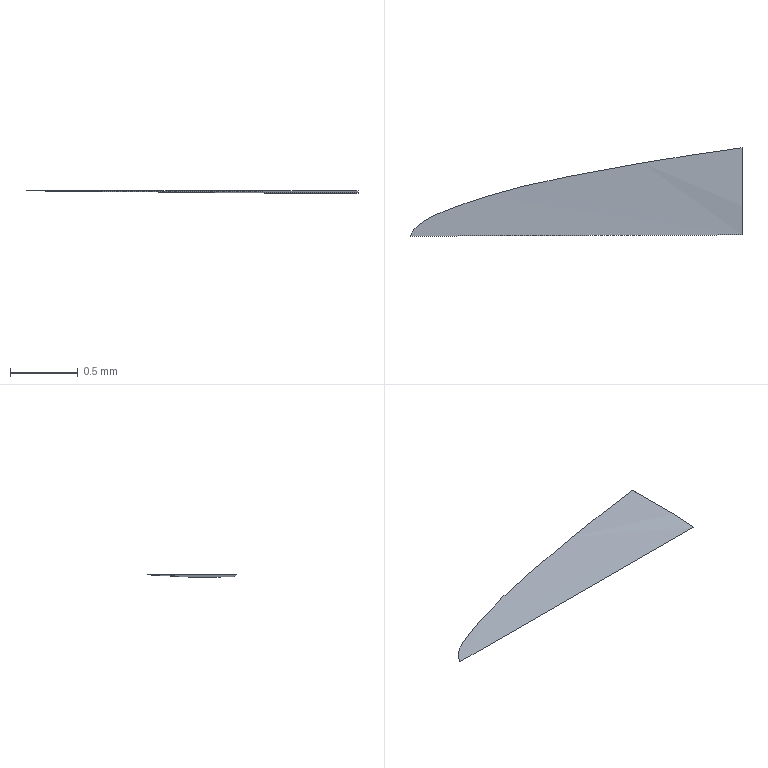Part | NX | features solid 2 | 1 solid | 3 faces | box 2.456 x 0.6536 x 0.02412 mm | volume 0.007379 mm3 | plane 2 | spline 1
STEP:
#1=CARTESIAN_POINT('',(202.544,-449.196,-62.));
#2=VERTEX_POINT('',#1);
#3=CARTESIAN_POINT('',(205.,-449.187,-62.012));
#4=VERTEX_POINT('',#3);
#5=CARTESIAN_POINT('',(202.544,-449.194,-62.));
#6=CARTESIAN_POINT('',(203.363,-449.192,-62.));
#7=CARTESIAN_POINT('',(204.181,-449.189,-62.));
#8=CARTESIAN_POINT('',(205.,-449.187,-62.));
#9=B_SPLINE_CURVE_WITH_KNOTS('',3,(#5,#6,#7,#8),.UNSPECIFIED.,.F.,.F.,(4,4),(0.,1.),.UNSPECIFIED.);
#10=EDGE_CURVE('',#2,#4,#9,.T.);
#11=ORIENTED_EDGE('',*,*,#10,.F.);
#12=CARTESIAN_POINT('',(205.,-448.543,-62.));
#13=VERTEX_POINT('',#12);
#14=CARTESIAN_POINT('',(202.544,-449.198,-62.));
#15=CARTESIAN_POINT('',(202.59,-449.098,-62.));
#16=CARTESIAN_POINT('',(202.806,-449.005,-62.));
#17=CARTESIAN_POINT('',(203.2,-448.864,-62.));
#18=CARTESIAN_POINT('',(203.942,-448.701,-62.));
#19=CARTESIAN_POINT('',(204.575,-448.601,-62.));
#20=CARTESIAN_POINT('',(205.,-448.543,-62.));
#21=B_SPLINE_CURVE_WITH_KNOTS('',3,(#14,#15,#16,#17,#18,#19,#20),.UNSPECIFIED.,.F.,.F.,(4,1,1,1,4),(0.,0.0003242,0.0006485,0.001297,0.002594),.UNSPECIFIED.);
#22=EDGE_CURVE('',#13,#2,#21,.F.);
#23=ORIENTED_EDGE('',*,*,#22,.F.);
#24=CARTESIAN_POINT('',(205.,-449.187,-62.024));
#25=CARTESIAN_POINT('',(205.,-448.971,-62.023));
#26=CARTESIAN_POINT('',(205.,-448.756,-62.015));
#27=CARTESIAN_POINT('',(205.,-448.543,-62.));
#28=B_SPLINE_CURVE_WITH_KNOTS('',3,(#24,#25,#26,#27),.UNSPECIFIED.,.F.,.F.,(4,4),(0.,0.0006386),.UNSPECIFIED.);
#29=EDGE_CURVE('',#4,#13,#28,.T.);
#30=ORIENTED_EDGE('',*,*,#29,.F.);
#31=EDGE_LOOP('',(#11,#23,#30));
#32=FACE_BOUND('',#31,.T.);
#33=CARTESIAN_POINT('',(205.015,-448.539,-62.));
#34=CARTESIAN_POINT('',(205.015,-448.669,-62.009));
#35=CARTESIAN_POINT('',(205.015,-448.8,-62.016));
#36=CARTESIAN_POINT('',(205.016,-448.93,-62.021));
#37=CARTESIAN_POINT('',(205.016,-449.061,-62.024));
#38=CARTESIAN_POINT('',(205.016,-449.191,-62.024));
#39=CARTESIAN_POINT('',(204.393,-448.54,-61.994));
#40=CARTESIAN_POINT('',(204.393,-448.671,-62.003));
#41=CARTESIAN_POINT('',(204.393,-448.801,-62.01));
#42=CARTESIAN_POINT('',(204.394,-448.932,-62.015));
#43=CARTESIAN_POINT('',(204.394,-449.062,-62.018));
#44=CARTESIAN_POINT('',(204.394,-449.193,-62.018));
#45=CARTESIAN_POINT('',(203.771,-448.542,-61.988));
#46=CARTESIAN_POINT('',(203.771,-448.672,-61.997));
#47=CARTESIAN_POINT('',(203.772,-448.803,-62.004));
#48=CARTESIAN_POINT('',(203.772,-448.933,-62.009));
#49=CARTESIAN_POINT('',(203.772,-449.064,-62.012));
#50=CARTESIAN_POINT('',(203.773,-449.195,-62.012));
#51=CARTESIAN_POINT('',(203.149,-448.544,-61.982));
#52=CARTESIAN_POINT('',(203.149,-448.674,-61.991));
#53=CARTESIAN_POINT('',(203.15,-448.804,-61.998));
#54=CARTESIAN_POINT('',(203.15,-448.935,-62.003));
#55=CARTESIAN_POINT('',(203.15,-449.066,-62.006));
#56=CARTESIAN_POINT('',(203.151,-449.196,-62.006));
#57=CARTESIAN_POINT('',(202.527,-448.545,-61.975));
#58=CARTESIAN_POINT('',(202.528,-448.676,-61.985));
#59=CARTESIAN_POINT('',(202.528,-448.806,-61.992));
#60=CARTESIAN_POINT('',(202.528,-448.937,-61.996));
#61=CARTESIAN_POINT('',(202.528,-449.067,-61.999));
#62=CARTESIAN_POINT('',(202.529,-449.198,-62.));
#63=B_SPLINE_SURFACE_WITH_KNOTS('',4,5,((#33,#34,#35,#36,#37,#38),(#39,#40,#41,#42,#43,#44),(#45,#46,#47,#48,#49,#50),(#51,#52,#53,#54,#55,#56),(#57,#58,#59,#60,#61,#62)),.UNSPECIFIED.,.F.,.F.,.F.,(5,5),(6,6),(0.7993,0.8627),(0.9553,1.),.PIECEWISE_BEZIER_KNOTS.);
#64=ADVANCED_FACE('',(#32),#63,.F.);
#65=CARTESIAN_POINT('',(205.,-469.337,-62.));
#66=DIRECTION('',(0.,1.,0.));
#67=VECTOR('',#66,1000.);
#68=LINE('',#65,#67);
#69=EDGE_CURVE('',#4,#13,#68,.T.);
#70=ORIENTED_EDGE('',*,*,#69,.F.);
#71=ORIENTED_EDGE('',*,*,#29,.T.);
#72=EDGE_LOOP('',(#70,#71));
#73=FACE_BOUND('',#72,.T.);
#74=CARTESIAN_POINT('',(205.,-469.337,-200.));
#75=DIRECTION('',(1.,0.,0.));
#76=DIRECTION('',(0.,0.,-1.));
#77=AXIS2_PLACEMENT_3D('',#74,#75,#76);
#78=PLANE('',#77);
#79=ADVANCED_FACE('',(#73),#78,.T.);
#80=ORIENTED_EDGE('',*,*,#10,.T.);
#81=ORIENTED_EDGE('',*,*,#69,.T.);
#82=ORIENTED_EDGE('',*,*,#22,.T.);
#83=EDGE_LOOP('',(#80,#81,#82));
#84=FACE_BOUND('',#83,.T.);
#85=CARTESIAN_POINT('',(190.5,-385.,-62.));
#86=DIRECTION('',(0.,0.,-1.));
#87=DIRECTION('',(-1.,0.,0.));
#88=AXIS2_PLACEMENT_3D('',#85,#86,#87);
#89=PLANE('',#88);
#90=ADVANCED_FACE('',(#84),#89,.F.);
#91=CLOSED_SHELL('',(#64,#79,#90));
#92=MANIFOLD_SOLID_BREP('',#91);
#93=(LENGTH_UNIT()NAMED_UNIT(*)SI_UNIT(.MILLI.,.METRE.));
#94=UNCERTAINTY_MEASURE_WITH_UNIT(LENGTH_MEASURE(0.08203),#93,'','');
#95=(NAMED_UNIT(*)PLANE_ANGLE_UNIT()SI_UNIT($,.RADIAN.));
#96=(NAMED_UNIT(*)SI_UNIT($,.STERADIAN.)SOLID_ANGLE_UNIT());
#97=(GEOMETRIC_REPRESENTATION_CONTEXT(3)GLOBAL_UNCERTAINTY_ASSIGNED_CONTEXT((#94))GLOBAL_UNIT_ASSIGNED_CONTEXT((#93,#95,#96))REPRESENTATION_CONTEXT('',''));
#98=ADVANCED_BREP_SHAPE_REPRESENTATION('',(#92),#97);